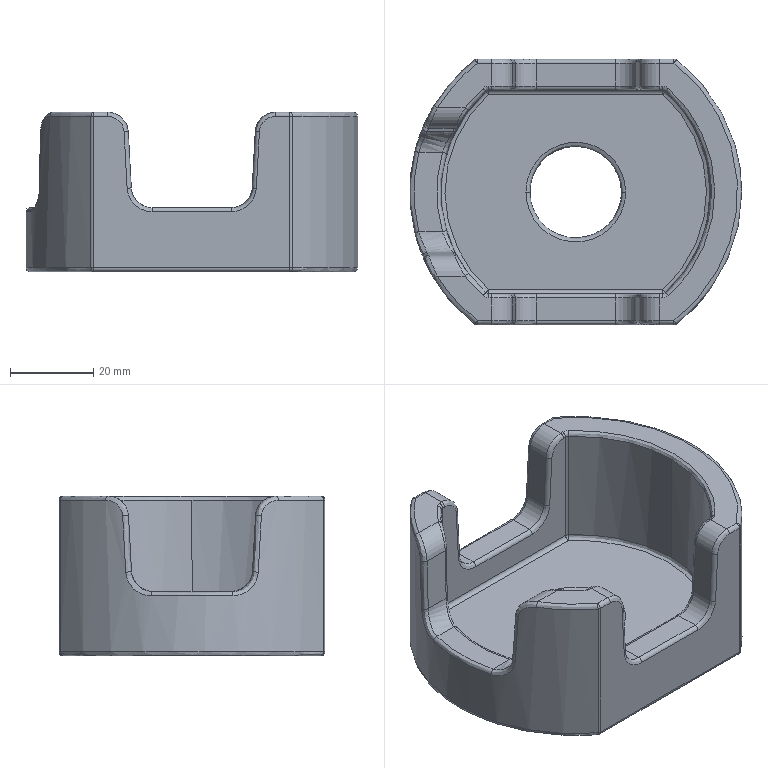Part | SolidWorks | features BaseBody 1 | 1 solid | 130 faces | box 80 x 64 x 38.5 mm | volume 66365 mm3 | cylinder 50 | spline 50 | plane 18 | sphere 12 | commonest cylinder face diameters 2 x32 10 x10 65 x3 80 x3 22 x2